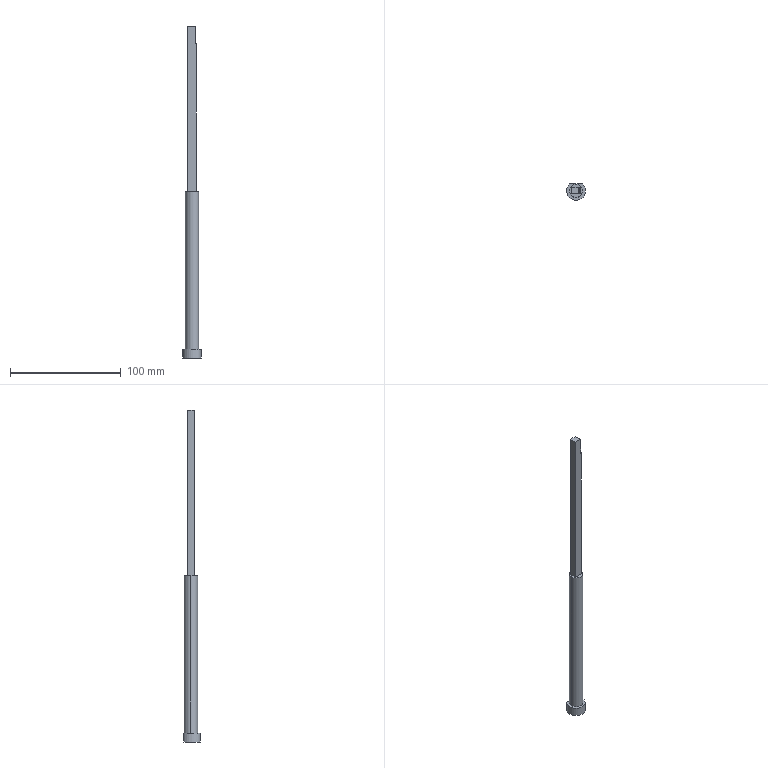Part | Creo | 1 solid | 15 faces | box 17 x 15 x 299.128 mm | volume 24813 mm3 | plane 10 | cylinder 3 | cone 1 | torus 1 | commonest cylinder face diameters 12 x2 17 x1
STEP:
#1=CARTESIAN_POINT('',(-72.523,-7.5,-296.));
#2=VERTEX_POINT('',#1);
#3=CARTESIAN_POINT('',(-69.5,-14.,-296.));
#4=VERTEX_POINT('',#3);
#5=CARTESIAN_POINT('',(-78.,-14.,-296.));
#6=DIRECTION('',(0.,0.,-1.));
#7=DIRECTION('',(0.6444,0.7647,0.));
#8=AXIS2_PLACEMENT_3D('',#5,#6,#7);
#9=CIRCLE('',#8,8.5);
#10=EDGE_CURVE('',#2,#4,#9,.T.);
#11=ORIENTED_EDGE('',*,*,#10,.F.);
#12=CARTESIAN_POINT('',(-83.477,-7.5,-296.));
#13=VERTEX_POINT('',#12);
#14=CARTESIAN_POINT('',(-72.523,-7.5,-296.));
#15=DIRECTION('',(-1.,0.,0.));
#16=VECTOR('',#15,10.954);
#17=LINE('',#14,#16);
#18=EDGE_CURVE('',#2,#13,#17,.T.);
#19=ORIENTED_EDGE('',*,*,#18,.T.);
#20=CARTESIAN_POINT('',(-78.,-14.,-296.));
#21=DIRECTION('',(0.,0.,-1.));
#22=DIRECTION('',(1.,0.,0.));
#23=AXIS2_PLACEMENT_3D('',#20,#21,#22);
#24=CIRCLE('',#23,8.5);
#25=EDGE_CURVE('',#4,#13,#24,.T.);
#26=ORIENTED_EDGE('',*,*,#25,.F.);
#27=EDGE_LOOP('',(#11,#19,#26));
#28=FACE_OUTER_BOUND('',#27,.F.);
#29=CARTESIAN_POINT('',(10.,-1.005,-296.));
#30=DIRECTION('',(0.,0.,1.));
#31=DIRECTION('',(0.,-1.,0.));
#32=AXIS2_PLACEMENT_3D('',#29,#30,#31);
#33=PLANE('',#32);
#34=ADVANCED_FACE('',(#28),#33,.F.);
#35=CARTESIAN_POINT('',(-83.477,-7.5,-288.));
#36=VERTEX_POINT('',#35);
#37=CARTESIAN_POINT('',(-83.477,-7.5,-288.));
#38=DIRECTION('',(0.,0.,-1.));
#39=VECTOR('',#38,8.);
#40=LINE('',#37,#39);
#41=EDGE_CURVE('',#36,#13,#40,.T.);
#42=ORIENTED_EDGE('',*,*,#41,.F.);
#43=CARTESIAN_POINT('',(-69.5,-14.,-288.));
#44=VERTEX_POINT('',#43);
#45=CARTESIAN_POINT('',(-78.,-14.,-288.));
#46=DIRECTION('',(0.,0.,1.));
#47=DIRECTION('',(-0.6444,0.7647,0.));
#48=AXIS2_PLACEMENT_3D('',#45,#46,#47);
#49=CIRCLE('',#48,8.5);
#50=EDGE_CURVE('',#36,#44,#49,.T.);
#51=ORIENTED_EDGE('',*,*,#50,.T.);
#52=CARTESIAN_POINT('',(-72.523,-7.5,-288.));
#53=VERTEX_POINT('',#52);
#54=CARTESIAN_POINT('',(-78.,-14.,-288.));
#55=DIRECTION('',(0.,0.,1.));
#56=DIRECTION('',(1.,0.,0.));
#57=AXIS2_PLACEMENT_3D('',#54,#55,#56);
#58=CIRCLE('',#57,8.5);
#59=EDGE_CURVE('',#44,#53,#58,.T.);
#60=ORIENTED_EDGE('',*,*,#59,.T.);
#61=CARTESIAN_POINT('',(-72.523,-7.5,-296.));
#62=DIRECTION('',(0.,0.,1.));
#63=VECTOR('',#62,8.);
#64=LINE('',#61,#63);
#65=EDGE_CURVE('',#2,#53,#64,.T.);
#66=ORIENTED_EDGE('',*,*,#65,.F.);
#67=ORIENTED_EDGE('',*,*,#10,.T.);
#68=ORIENTED_EDGE('',*,*,#25,.T.);
#69=EDGE_LOOP('',(#42,#51,#60,#66,#67,#68));
#70=FACE_OUTER_BOUND('',#69,.F.);
#71=CARTESIAN_POINT('',(-78.,-14.,-288.));
#72=DIRECTION('',(0.,0.,-1.));
#73=DIRECTION('',(1.,0.,0.));
#74=AXIS2_PLACEMENT_3D('',#71,#72,#73);
#75=CYLINDRICAL_SURFACE('',#74,8.5);
#76=ADVANCED_FACE('',(#70),#75,.T.);
#77=ORIENTED_EDGE('',*,*,#41,.T.);
#78=ORIENTED_EDGE('',*,*,#18,.F.);
#79=ORIENTED_EDGE('',*,*,#65,.T.);
#80=CARTESIAN_POINT('',(-83.477,-7.5,-288.));
#81=DIRECTION('',(1.,0.,0.));
#82=VECTOR('',#81,10.954);
#83=LINE('',#80,#82);
#84=EDGE_CURVE('',#36,#53,#83,.T.);
#85=ORIENTED_EDGE('',*,*,#84,.F.);
#86=EDGE_LOOP('',(#77,#78,#79,#85));
#87=FACE_OUTER_BOUND('',#86,.F.);
#88=CARTESIAN_POINT('',(-78.,-7.5,-296.));
#89=DIRECTION('',(0.,-1.,0.));
#90=DIRECTION('',(0.,0.,1.));
#91=AXIS2_PLACEMENT_3D('',#88,#89,#90);
#92=PLANE('',#91);
#93=ADVANCED_FACE('',(#87),#92,.F.);
#94=ORIENTED_EDGE('',*,*,#50,.F.);
#95=ORIENTED_EDGE('',*,*,#84,.T.);
#96=ORIENTED_EDGE('',*,*,#59,.F.);
#97=EDGE_LOOP('',(#94,#95,#96));
#98=FACE_OUTER_BOUND('',#97,.F.);
#99=CARTESIAN_POINT('',(-84.,-14.,-288.));
#100=VERTEX_POINT('',#99);
#101=CARTESIAN_POINT('',(-72.,-14.,-288.));
#102=VERTEX_POINT('',#101);
#103=CARTESIAN_POINT('',(-78.,-14.,-288.));
#104=DIRECTION('',(0.,0.,-1.));
#105=DIRECTION('',(-1.,0.,0.));
#106=AXIS2_PLACEMENT_3D('',#103,#104,#105);
#107=CIRCLE('',#106,6.);
#108=EDGE_CURVE('',#100,#102,#107,.T.);
#109=ORIENTED_EDGE('',*,*,#108,.F.);
#110=CARTESIAN_POINT('',(-78.,-14.,-288.));
#111=DIRECTION('',(0.,0.,-1.));
#112=DIRECTION('',(1.,0.,0.));
#113=AXIS2_PLACEMENT_3D('',#110,#111,#112);
#114=CIRCLE('',#113,6.);
#115=EDGE_CURVE('',#102,#100,#114,.T.);
#116=ORIENTED_EDGE('',*,*,#115,.F.);
#117=EDGE_LOOP('',(#109,#116));
#118=FACE_BOUND('',#117,.F.);
#119=CARTESIAN_POINT('',(-78.,-14.,-288.));
#120=DIRECTION('',(0.,0.,-1.));
#121=DIRECTION('',(1.,0.,0.));
#122=AXIS2_PLACEMENT_3D('',#119,#120,#121);
#123=PLANE('',#122);
#124=ADVANCED_FACE('',(#98,#118),#123,.F.);
#125=CARTESIAN_POINT('',(-72.,-14.,-146.));
#126=VERTEX_POINT('',#125);
#127=CARTESIAN_POINT('',(-84.,-14.,-146.));
#128=VERTEX_POINT('',#127);
#129=CARTESIAN_POINT('',(-78.,-14.,-146.));
#130=DIRECTION('',(0.,0.,1.));
#131=DIRECTION('',(1.,0.,0.));
#132=AXIS2_PLACEMENT_3D('',#129,#130,#131);
#133=CIRCLE('',#132,6.);
#134=EDGE_CURVE('',#126,#128,#133,.T.);
#135=ORIENTED_EDGE('',*,*,#134,.T.);
#136=CARTESIAN_POINT('',(-84.,-14.,-288.));
#137=DIRECTION('',(0.,0.,1.));
#138=VECTOR('',#137,142.);
#139=LINE('',#136,#138);
#140=EDGE_CURVE('',#100,#128,#139,.T.);
#141=ORIENTED_EDGE('',*,*,#140,.F.);
#142=ORIENTED_EDGE('',*,*,#108,.T.);
#143=CARTESIAN_POINT('',(-72.,-14.,-288.));
#144=DIRECTION('',(0.,0.,1.));
#145=VECTOR('',#144,142.);
#146=LINE('',#143,#145);
#147=EDGE_CURVE('',#102,#126,#146,.T.);
#148=ORIENTED_EDGE('',*,*,#147,.T.);
#149=EDGE_LOOP('',(#135,#141,#142,#148));
#150=FACE_OUTER_BOUND('',#149,.F.);
#151=CARTESIAN_POINT('',(-78.,-14.,-153.));
#152=DIRECTION('',(0.,0.,1.));
#153=DIRECTION('',(-1.,0.,0.));
#154=AXIS2_PLACEMENT_3D('',#151,#152,#153);
#155=CYLINDRICAL_SURFACE('',#154,6.);
#156=ADVANCED_FACE('',(#150),#155,.T.);
#157=CARTESIAN_POINT('',(-78.,-14.,-146.));
#158=DIRECTION('',(0.,0.,1.));
#159=DIRECTION('',(-1.,0.,0.));
#160=AXIS2_PLACEMENT_3D('',#157,#158,#159);
#161=CIRCLE('',#160,6.);
#162=EDGE_CURVE('',#128,#126,#161,.T.);
#163=ORIENTED_EDGE('',*,*,#162,.F.);
#164=ORIENTED_EDGE('',*,*,#134,.F.);
#165=EDGE_LOOP('',(#163,#164));
#166=FACE_OUTER_BOUND('',#165,.F.);
#167=CARTESIAN_POINT('',(-74.,-11.,-146.));
#168=VERTEX_POINT('',#167);
#169=CARTESIAN_POINT('',(-74.,-17.,-146.));
#170=VERTEX_POINT('',#169);
#171=CARTESIAN_POINT('',(-74.,-11.,-146.));
#172=DIRECTION('',(0.,-1.,0.));
#173=VECTOR('',#172,6.);
#174=LINE('',#171,#173);
#175=EDGE_CURVE('',#168,#170,#174,.T.);
#176=ORIENTED_EDGE('',*,*,#175,.F.);
#177=CARTESIAN_POINT('',(-82.,-11.,-146.));
#178=VERTEX_POINT('',#177);
#179=CARTESIAN_POINT('',(-82.,-11.,-146.));
#180=DIRECTION('',(1.,0.,0.));
#181=VECTOR('',#180,8.);
#182=LINE('',#179,#181);
#183=EDGE_CURVE('',#178,#168,#182,.T.);
#184=ORIENTED_EDGE('',*,*,#183,.F.);
#185=CARTESIAN_POINT('',(-82.,-17.,-146.));
#186=VERTEX_POINT('',#185);
#187=CARTESIAN_POINT('',(-82.,-17.,-146.));
#188=DIRECTION('',(0.,1.,0.));
#189=VECTOR('',#188,6.);
#190=LINE('',#187,#189);
#191=EDGE_CURVE('',#186,#178,#190,.T.);
#192=ORIENTED_EDGE('',*,*,#191,.F.);
#193=CARTESIAN_POINT('',(-74.,-17.,-146.));
#194=DIRECTION('',(-1.,0.,0.));
#195=VECTOR('',#194,8.);
#196=LINE('',#193,#195);
#197=EDGE_CURVE('',#170,#186,#196,.T.);
#198=ORIENTED_EDGE('',*,*,#197,.F.);
#199=EDGE_LOOP('',(#176,#184,#192,#198));
#200=FACE_BOUND('',#199,.F.);
#201=CARTESIAN_POINT('',(-78.,-14.,-146.));
#202=DIRECTION('',(0.,0.,-1.));
#203=DIRECTION('',(1.,0.,0.));
#204=AXIS2_PLACEMENT_3D('',#201,#202,#203);
#205=PLANE('',#204);
#206=ADVANCED_FACE('',(#166,#200),#205,.F.);
#207=ORIENTED_EDGE('',*,*,#162,.T.);
#208=ORIENTED_EDGE('',*,*,#147,.F.);
#209=ORIENTED_EDGE('',*,*,#115,.T.);
#210=ORIENTED_EDGE('',*,*,#140,.T.);
#211=EDGE_LOOP('',(#207,#208,#209,#210));
#212=FACE_OUTER_BOUND('',#211,.F.);
#213=CARTESIAN_POINT('',(-78.,-14.,-153.));
#214=DIRECTION('',(0.,0.,1.));
#215=DIRECTION('',(-1.,0.,0.));
#216=AXIS2_PLACEMENT_3D('',#213,#214,#215);
#217=CYLINDRICAL_SURFACE('',#216,6.);
#218=ADVANCED_FACE('',(#212),#217,.T.);
#219=CARTESIAN_POINT('',(-74.,-11.,-12.688));
#220=VERTEX_POINT('',#219);
#221=CARTESIAN_POINT('',(-74.,-11.,-12.688));
#222=DIRECTION('',(0.,0.,-1.));
#223=VECTOR('',#222,133.312);
#224=LINE('',#221,#223);
#225=EDGE_CURVE('',#220,#168,#224,.T.);
#226=ORIENTED_EDGE('',*,*,#225,.T.);
#227=ORIENTED_EDGE('',*,*,#175,.T.);
#228=CARTESIAN_POINT('',(-74.,-17.,-12.688));
#229=VERTEX_POINT('',#228);
#230=CARTESIAN_POINT('',(-74.,-17.,-12.688));
#231=DIRECTION('',(0.,0.,-1.));
#232=VECTOR('',#231,133.312);
#233=LINE('',#230,#232);
#234=EDGE_CURVE('',#229,#170,#233,.T.);
#235=ORIENTED_EDGE('',*,*,#234,.F.);
#236=CARTESIAN_POINT('',(-74.,-17.,-12.688));
#237=DIRECTION('',(0.,1.,0.));
#238=VECTOR('',#237,6.);
#239=LINE('',#236,#238);
#240=EDGE_CURVE('',#229,#220,#239,.T.);
#241=ORIENTED_EDGE('',*,*,#240,.T.);
#242=EDGE_LOOP('',(#226,#227,#235,#241));
#243=FACE_OUTER_BOUND('',#242,.F.);
#244=CARTESIAN_POINT('',(-74.,-13.,-15.));
#245=DIRECTION('',(1.,0.,0.));
#246=DIRECTION('',(0.,0.,1.));
#247=AXIS2_PLACEMENT_3D('',#244,#245,#246);
#248=PLANE('',#247);
#249=ADVANCED_FACE('',(#243),#248,.T.);
#250=CARTESIAN_POINT('',(-75.286,-11.,2.634));
#251=VERTEX_POINT('',#250);
#252=CARTESIAN_POINT('',(-75.018,-11.,-12.688));
#253=VERTEX_POINT('',#252);
#254=CARTESIAN_POINT('',(-75.286,-11.,2.634));
#255=DIRECTION('',(0.01746,-0.000000774,-0.9998));
#256=VECTOR('',#255,15.324);
#257=LINE('',#254,#256);
#258=EDGE_CURVE('',#251,#253,#257,.T.);
#259=ORIENTED_EDGE('',*,*,#258,.F.);
#260=CARTESIAN_POINT('',(-75.788,-11.,3.128));
#261=VERTEX_POINT('',#260);
#262=CARTESIAN_POINT('',(-75.286,-11.,2.634));
#263=CARTESIAN_POINT('',(-75.287,-11.,2.728));
#264=CARTESIAN_POINT('',(-75.335,-11.,2.89));
#265=CARTESIAN_POINT('',(-75.531,-11.,3.082));
#266=CARTESIAN_POINT('',(-75.694,-11.,3.128));
#267=CARTESIAN_POINT('',(-75.788,-11.,3.128));
#268=B_SPLINE_CURVE_WITH_KNOTS('',3,(#262,#263,#264,#265,#266,#267),.UNSPECIFIED.,.F.,.F.,(4,1,1,4),(0.,0.3333,0.6667,1.),.UNSPECIFIED.);
#269=EDGE_CURVE('',#251,#261,#268,.T.);
#270=ORIENTED_EDGE('',*,*,#269,.T.);
#271=CARTESIAN_POINT('',(-82.,-11.,3.128));
#272=VERTEX_POINT('',#271);
#273=CARTESIAN_POINT('',(-75.788,-11.,3.128));
#274=DIRECTION('',(-1.,-0.000001656,-0.000000371));
#275=VECTOR('',#274,6.212);
#276=LINE('',#273,#275);
#277=EDGE_CURVE('',#261,#272,#276,.T.);
#278=ORIENTED_EDGE('',*,*,#277,.T.);
#279=CARTESIAN_POINT('',(-82.,-11.,3.128));
#280=DIRECTION('',(0.,0.,-1.));
#281=VECTOR('',#280,149.128);
#282=LINE('',#279,#281);
#283=EDGE_CURVE('',#272,#178,#282,.T.);
#284=ORIENTED_EDGE('',*,*,#283,.T.);
#285=ORIENTED_EDGE('',*,*,#183,.T.);
#286=ORIENTED_EDGE('',*,*,#225,.F.);
#287=CARTESIAN_POINT('',(-74.,-11.,-12.688));
#288=DIRECTION('',(-1.,-0.00001082,-0.000006855));
#289=VECTOR('',#288,1.018);
#290=LINE('',#287,#289);
#291=EDGE_CURVE('',#220,#253,#290,.T.);
#292=ORIENTED_EDGE('',*,*,#291,.T.);
#293=EDGE_LOOP('',(#259,#270,#278,#284,#285,#286,#292));
#294=FACE_OUTER_BOUND('',#293,.F.);
#295=CARTESIAN_POINT('',(-78.,-11.,-15.));
#296=DIRECTION('',(0.,1.,0.));
#297=DIRECTION('',(0.,0.,-1.));
#298=AXIS2_PLACEMENT_3D('',#295,#296,#297);
#299=PLANE('',#298);
#300=ADVANCED_FACE('',(#294),#299,.T.);
#301=CARTESIAN_POINT('',(-74.807,-17.,-12.688));
#302=VERTEX_POINT('',#301);
#303=CARTESIAN_POINT('',(-75.074,-17.,2.634));
#304=VERTEX_POINT('',#303);
#305=CARTESIAN_POINT('',(-74.807,-17.,-12.688));
#306=DIRECTION('',(-0.01747,0.000002896,0.9998));
#307=VECTOR('',#306,15.324);
#308=LINE('',#305,#307);
#309=EDGE_CURVE('',#302,#304,#308,.T.);
#310=ORIENTED_EDGE('',*,*,#309,.T.);
#311=CARTESIAN_POINT('',(314.396,-0.2635,2.703));
#312=DIRECTION('',(-0.0001773,-0.000005309,1.));
#313=DIRECTION('',(-0.9996,-0.02754,-0.0001774));
#314=AXIS2_PLACEMENT_3D('',#311,#312,#313);
#315=CIRCLE('',#314,389.83);
#316=EDGE_CURVE('',#251,#304,#315,.T.);
#317=ORIENTED_EDGE('',*,*,#316,.F.);
#318=ORIENTED_EDGE('',*,*,#258,.T.);
#319=CARTESIAN_POINT('',(-75.018,-11.,-12.688));
#320=CARTESIAN_POINT('',(-75.,-11.665,-12.688));
#321=CARTESIAN_POINT('',(-74.959,-12.995,-12.688));
#322=CARTESIAN_POINT('',(-74.889,-14.995,-12.688));
#323=CARTESIAN_POINT('',(-74.835,-16.331,-12.688));
#324=CARTESIAN_POINT('',(-74.807,-17.,-12.688));
#325=B_SPLINE_CURVE_WITH_KNOTS('',3,(#319,#320,#321,#322,#323,#324),.UNSPECIFIED.,.F.,.F.,(4,1,1,4),(0.,0.3333,0.6667,1.),.UNSPECIFIED.);
#326=EDGE_CURVE('',#253,#302,#325,.T.);
#327=ORIENTED_EDGE('',*,*,#326,.T.);
#328=EDGE_LOOP('',(#310,#317,#318,#327));
#329=FACE_OUTER_BOUND('',#328,.F.);
#330=CARTESIAN_POINT('',(314.397,-0.2635,-4.959));
#331=DIRECTION('',(-0.0001773,-0.000005309,1.));
#332=DIRECTION('',(-0.9996,-0.02754,-0.0001774));
#333=AXIS2_PLACEMENT_3D('',#330,#331,#332);
#334=CONICAL_SURFACE('',#333,389.698,0.9898);
#335=ADVANCED_FACE('',(#329),#334,.F.);
#336=ORIENTED_EDGE('',*,*,#234,.T.);
#337=ORIENTED_EDGE('',*,*,#197,.T.);
#338=CARTESIAN_POINT('',(-82.,-17.,3.128));
#339=VERTEX_POINT('',#338);
#340=CARTESIAN_POINT('',(-82.,-17.,3.128));
#341=DIRECTION('',(0.,0.,-1.));
#342=VECTOR('',#341,149.128);
#343=LINE('',#340,#342);
#344=EDGE_CURVE('',#339,#186,#343,.T.);
#345=ORIENTED_EDGE('',*,*,#344,.F.);
#346=CARTESIAN_POINT('',(-75.577,-17.,3.128));
#347=VERTEX_POINT('',#346);
#348=CARTESIAN_POINT('',(-82.,-17.,3.128));
#349=DIRECTION('',(1.,0.00000717,0.000000749));
#350=VECTOR('',#349,6.423);
#351=LINE('',#348,#350);
#352=EDGE_CURVE('',#339,#347,#351,.T.);
#353=ORIENTED_EDGE('',*,*,#352,.T.);
#354=CARTESIAN_POINT('',(-75.483,-17.,3.127));
#355=CARTESIAN_POINT('',(-75.32,-17.,3.082));
#356=CARTESIAN_POINT('',(-75.123,-17.,2.89));
#357=CARTESIAN_POINT('',(-75.076,-17.,2.728));
#358=CARTESIAN_POINT('',(-75.074,-17.,2.634));
#359=B_SPLINE_CURVE_WITH_KNOTS('',3,(#346,#354,#355,#356,#357,#358),.UNSPECIFIED.,.F.,.F.,(4,1,1,4),(0.,0.3333,0.6667,1.),.UNSPECIFIED.);
#360=EDGE_CURVE('',#347,#304,#359,.T.);
#361=ORIENTED_EDGE('',*,*,#360,.T.);
#362=ORIENTED_EDGE('',*,*,#309,.F.);
#363=CARTESIAN_POINT('',(-74.807,-17.,-12.688));
#364=DIRECTION('',(1.,0.0000213,0.000008654));
#365=VECTOR('',#364,0.8065);
#366=LINE('',#363,#365);
#367=EDGE_CURVE('',#302,#229,#366,.T.);
#368=ORIENTED_EDGE('',*,*,#367,.T.);
#369=EDGE_LOOP('',(#336,#337,#345,#353,#361,#362,#368));
#370=FACE_OUTER_BOUND('',#369,.F.);
#371=CARTESIAN_POINT('',(-78.,-17.,-15.));
#372=DIRECTION('',(0.,-1.,0.));
#373=DIRECTION('',(0.,0.,1.));
#374=AXIS2_PLACEMENT_3D('',#371,#372,#373);
#375=PLANE('',#374);
#376=ADVANCED_FACE('',(#370),#375,.T.);
#377=ORIENTED_EDGE('',*,*,#344,.T.);
#378=ORIENTED_EDGE('',*,*,#191,.T.);
#379=ORIENTED_EDGE('',*,*,#283,.F.);
#380=CARTESIAN_POINT('',(-82.,-11.,3.128));
#381=DIRECTION('',(0.,-1.,0.));
#382=VECTOR('',#381,6.);
#383=LINE('',#380,#382);
#384=EDGE_CURVE('',#272,#339,#383,.T.);
#385=ORIENTED_EDGE('',*,*,#384,.T.);
#386=EDGE_LOOP('',(#377,#378,#379,#385));
#387=FACE_OUTER_BOUND('',#386,.F.);
#388=CARTESIAN_POINT('',(-82.,-13.,-15.));
#389=DIRECTION('',(-1.,0.,0.));
#390=DIRECTION('',(0.,0.,-1.));
#391=AXIS2_PLACEMENT_3D('',#388,#389,#390);
#392=PLANE('',#391);
#393=ADVANCED_FACE('',(#387),#392,.T.);
#394=CARTESIAN_POINT('',(-75.577,-17.,3.128));
#395=CARTESIAN_POINT('',(-75.605,-16.333,3.128));
#396=CARTESIAN_POINT('',(-75.659,-15.,3.128));
#397=CARTESIAN_POINT('',(-75.729,-13.,3.128));
#398=CARTESIAN_POINT('',(-75.77,-11.667,3.128));
#399=CARTESIAN_POINT('',(-75.788,-11.,3.128));
#400=B_SPLINE_CURVE_WITH_KNOTS('',3,(#394,#395,#396,#397,#398,#399),.UNSPECIFIED.,.F.,.F.,(4,1,1,4),(0.,0.3333,0.6667,1.),.UNSPECIFIED.);
#401=EDGE_CURVE('',#347,#261,#400,.T.);
#402=ORIENTED_EDGE('',*,*,#401,.F.);
#403=ORIENTED_EDGE('',*,*,#352,.F.);
#404=ORIENTED_EDGE('',*,*,#384,.F.);
#405=ORIENTED_EDGE('',*,*,#277,.F.);
#406=EDGE_LOOP('',(#402,#403,#404,#405));
#407=FACE_OUTER_BOUND('',#406,.F.);
#408=CARTESIAN_POINT('',(-78.,-13.,3.128));
#409=DIRECTION('',(0.,0.,1.));
#410=DIRECTION('',(-1.,0.,0.));
#411=AXIS2_PLACEMENT_3D('',#408,#409,#410);
#412=PLANE('',#411);
#413=ADVANCED_FACE('',(#407),#412,.T.);
#414=ORIENTED_EDGE('',*,*,#316,.T.);
#415=ORIENTED_EDGE('',*,*,#360,.F.);
#416=ORIENTED_EDGE('',*,*,#401,.T.);
#417=ORIENTED_EDGE('',*,*,#269,.F.);
#418=EDGE_LOOP('',(#414,#415,#416,#417));
#419=FACE_OUTER_BOUND('',#418,.F.);
#420=CARTESIAN_POINT('',(316.393,-0.2099,2.456));
#421=DIRECTION('',(-0.0004294,-0.00001638,-1.));
#422=DIRECTION('',(-0.9983,-0.05774,0.0004296));
#423=AXIS2_PLACEMENT_3D('',#420,#421,#422);
#424=TOROIDAL_SURFACE('',#423,392.33,0.5029);
#425=ADVANCED_FACE('',(#419),#424,.T.);
#426=ORIENTED_EDGE('',*,*,#240,.F.);
#427=ORIENTED_EDGE('',*,*,#367,.F.);
#428=ORIENTED_EDGE('',*,*,#326,.F.);
#429=ORIENTED_EDGE('',*,*,#291,.F.);
#430=EDGE_LOOP('',(#426,#427,#428,#429));
#431=FACE_OUTER_BOUND('',#430,.F.);
#432=CARTESIAN_POINT('',(0.,0.,-12.688));
#433=DIRECTION('',(0.,0.,1.));
#434=DIRECTION('',(0.,1.,0.));
#435=AXIS2_PLACEMENT_3D('',#432,#433,#434);
#436=PLANE('',#435);
#437=ADVANCED_FACE('',(#431),#436,.T.);
#438=CLOSED_SHELL('',(#34,#76,#93,#124,#156,#206,#218,#249,#300,#335,#376,#393,#413,#425,#437));
#439=MANIFOLD_SOLID_BREP('',#438);
#440=(LENGTH_UNIT()NAMED_UNIT(*)SI_UNIT(.MILLI.,.METRE.));
#441=UNCERTAINTY_MEASURE_WITH_UNIT(LENGTH_MEASURE(0.03),#440,'','');
#442=(NAMED_UNIT(*)PLANE_ANGLE_UNIT()SI_UNIT($,.RADIAN.));
#443=PLANE_ANGLE_MEASURE_WITH_UNIT(PLANE_ANGLE_MEASURE(0.01745),#442);
#444=(CONVERSION_BASED_UNIT('DEGREE',#443)NAMED_UNIT(*)PLANE_ANGLE_UNIT());
#445=(NAMED_UNIT(*)SI_UNIT($,.STERADIAN.)SOLID_ANGLE_UNIT());
#446=(GEOMETRIC_REPRESENTATION_CONTEXT(3)GLOBAL_UNCERTAINTY_ASSIGNED_CONTEXT((#441))GLOBAL_UNIT_ASSIGNED_CONTEXT((#440,#444,#445))REPRESENTATION_CONTEXT('',''));
#447=ADVANCED_BREP_SHAPE_REPRESENTATION('',(#439),#446);